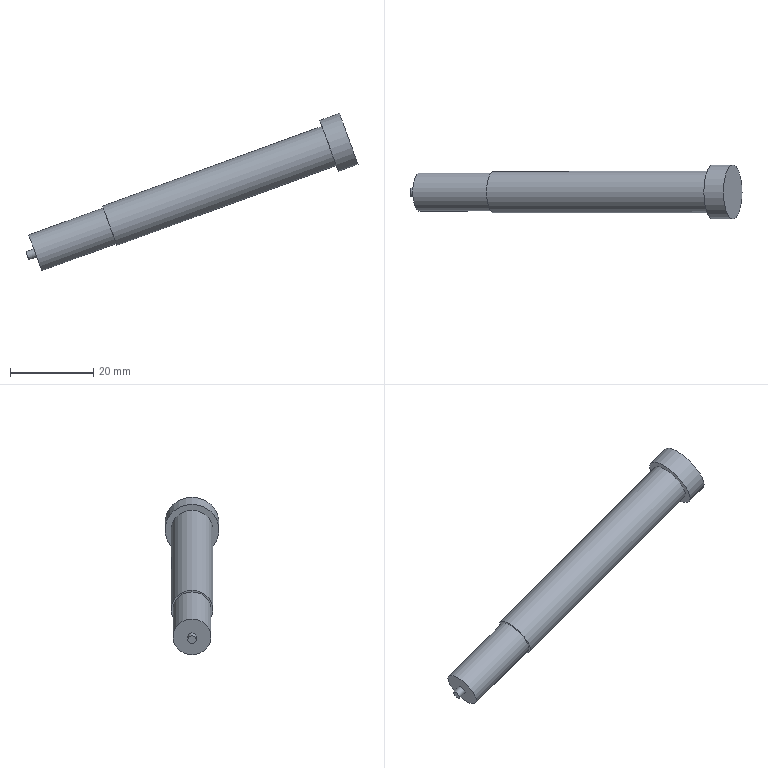Part | NX | features solid 2 | 1 solid | 9 faces | box 79.62 x 13 x 37.745 mm | volume 6304 mm3 | plane 5 | cylinder 4 | commonest cylinder face diameters 2 x1 9.1 x1 10 x1 13 x1
STEP:
#1=CARTESIAN_POINT('',(678.985,-306.988,36.091));
#2=VERTEX_POINT('',#1);
#3=CARTESIAN_POINT('',(680.695,-306.988,31.393));
#4=DIRECTION('',(-0.9397,0.000001517,-0.342));
#5=DIRECTION('',(-0.342,0.00000071,0.9397));
#6=AXIS2_PLACEMENT_3D('',#3,#4,#5);
#7=CIRCLE('',#6,5.);
#8=EDGE_CURVE('',#2,#2,#7,.T.);
#9=ORIENTED_EDGE('',*,*,#8,.F.);
#10=EDGE_LOOP('',(#9));
#11=FACE_BOUND('',#10,.T.);
#12=CARTESIAN_POINT('',(731.608,-306.989,55.244));
#13=VERTEX_POINT('',#12);
#14=CARTESIAN_POINT('',(733.318,-306.989,50.546));
#15=DIRECTION('',(-0.9397,0.000001517,-0.342));
#16=DIRECTION('',(-0.342,0.00000071,0.9397));
#17=AXIS2_PLACEMENT_3D('',#14,#15,#16);
#18=CIRCLE('',#17,5.);
#19=EDGE_CURVE('',#13,#13,#18,.T.);
#20=ORIENTED_EDGE('',*,*,#19,.T.);
#21=EDGE_LOOP('',(#20));
#22=FACE_BOUND('',#21,.T.);
#23=CARTESIAN_POINT('',(738.016,-306.989,52.256));
#24=DIRECTION('',(-0.9397,0.000001517,-0.342));
#25=DIRECTION('',(0.342,-0.00000071,-0.9397));
#26=AXIS2_PLACEMENT_3D('',#23,#24,#25);
#27=CYLINDRICAL_SURFACE('',#26,5.);
#28=ADVANCED_FACE('',(#11,#22),#27,.T.);
#29=CARTESIAN_POINT('',(679.139,-306.988,35.668));
#30=VERTEX_POINT('',#29);
#31=CARTESIAN_POINT('',(680.695,-306.988,31.393));
#32=DIRECTION('',(-0.9397,0.000001517,-0.342));
#33=DIRECTION('',(-0.342,0.00000071,0.9397));
#34=AXIS2_PLACEMENT_3D('',#31,#32,#33);
#35=CIRCLE('',#34,4.55);
#36=EDGE_CURVE('',#30,#30,#35,.T.);
#37=ORIENTED_EDGE('',*,*,#36,.F.);
#38=EDGE_LOOP('',(#37));
#39=FACE_BOUND('',#38,.T.);
#40=ORIENTED_EDGE('',*,*,#8,.T.);
#41=EDGE_LOOP('',(#40));
#42=FACE_BOUND('',#41,.T.);
#43=CARTESIAN_POINT('',(680.695,-306.988,31.393));
#44=DIRECTION('',(0.9397,-0.000001517,0.342));
#45=DIRECTION('',(-0.342,0.00000071,0.9397));
#46=AXIS2_PLACEMENT_3D('',#43,#44,#45);
#47=PLANE('',#46);
#48=ADVANCED_FACE('',(#39,#42),#47,.F.);
#49=CARTESIAN_POINT('',(731.095,-306.989,56.654));
#50=VERTEX_POINT('',#49);
#51=CARTESIAN_POINT('',(733.318,-306.989,50.546));
#52=DIRECTION('',(-0.9397,0.000001517,-0.342));
#53=DIRECTION('',(-0.342,0.00000071,0.9397));
#54=AXIS2_PLACEMENT_3D('',#51,#52,#53);
#55=CIRCLE('',#54,6.5);
#56=EDGE_CURVE('',#50,#50,#55,.T.);
#57=ORIENTED_EDGE('',*,*,#56,.T.);
#58=EDGE_LOOP('',(#57));
#59=FACE_BOUND('',#58,.T.);
#60=ORIENTED_EDGE('',*,*,#19,.F.);
#61=EDGE_LOOP('',(#60));
#62=FACE_BOUND('',#61,.T.);
#63=CARTESIAN_POINT('',(733.318,-306.989,50.546));
#64=DIRECTION('',(0.9397,-0.000001517,0.342));
#65=DIRECTION('',(-0.342,0.00000071,0.9397));
#66=AXIS2_PLACEMENT_3D('',#63,#64,#65);
#67=PLANE('',#66);
#68=ADVANCED_FACE('',(#59,#62),#67,.F.);
#69=ORIENTED_EDGE('',*,*,#56,.F.);
#70=EDGE_LOOP('',(#69));
#71=FACE_BOUND('',#70,.T.);
#72=CARTESIAN_POINT('',(735.793,-306.989,58.364));
#73=VERTEX_POINT('',#72);
#74=CARTESIAN_POINT('',(738.016,-306.989,52.256));
#75=DIRECTION('',(-0.9397,0.000001517,-0.342));
#76=DIRECTION('',(-0.342,0.00000071,0.9397));
#77=AXIS2_PLACEMENT_3D('',#74,#75,#76);
#78=CIRCLE('',#77,6.5);
#79=EDGE_CURVE('',#73,#73,#78,.T.);
#80=ORIENTED_EDGE('',*,*,#79,.T.);
#81=EDGE_LOOP('',(#80));
#82=FACE_BOUND('',#81,.T.);
#83=CARTESIAN_POINT('',(733.318,-306.989,50.546));
#84=DIRECTION('',(0.9397,-0.000001517,0.342));
#85=DIRECTION('',(-0.342,0.00000071,0.9397));
#86=AXIS2_PLACEMENT_3D('',#83,#84,#85);
#87=CYLINDRICAL_SURFACE('',#86,6.5);
#88=ADVANCED_FACE('',(#71,#82),#87,.T.);
#89=ORIENTED_EDGE('',*,*,#79,.F.);
#90=EDGE_LOOP('',(#89));
#91=FACE_BOUND('',#90,.T.);
#92=CARTESIAN_POINT('',(738.016,-306.989,52.256));
#93=DIRECTION('',(0.9397,-0.000001517,0.342));
#94=DIRECTION('',(-0.342,0.00000071,0.9397));
#95=AXIS2_PLACEMENT_3D('',#92,#93,#94);
#96=PLANE('',#95);
#97=ADVANCED_FACE('',(#91),#96,.T.);
#98=CARTESIAN_POINT('',(661.285,-306.988,29.17));
#99=VERTEX_POINT('',#98);
#100=CARTESIAN_POINT('',(662.841,-306.988,24.894));
#101=DIRECTION('',(-0.9397,0.000001517,-0.342));
#102=DIRECTION('',(-0.342,0.00000071,0.9397));
#103=AXIS2_PLACEMENT_3D('',#100,#101,#102);
#104=CIRCLE('',#103,4.55);
#105=EDGE_CURVE('',#99,#99,#104,.T.);
#106=ORIENTED_EDGE('',*,*,#105,.F.);
#107=EDGE_LOOP('',(#106));
#108=FACE_BOUND('',#107,.T.);
#109=ORIENTED_EDGE('',*,*,#36,.T.);
#110=EDGE_LOOP('',(#109));
#111=FACE_BOUND('',#110,.T.);
#112=CARTESIAN_POINT('',(662.841,-306.988,24.894));
#113=DIRECTION('',(0.9397,-0.000001517,0.342));
#114=DIRECTION('',(-0.342,0.00000071,0.9397));
#115=AXIS2_PLACEMENT_3D('',#112,#113,#114);
#116=CYLINDRICAL_SURFACE('',#115,4.55);
#117=ADVANCED_FACE('',(#108,#111),#116,.T.);
#118=CARTESIAN_POINT('',(662.499,-306.988,25.834));
#119=VERTEX_POINT('',#118);
#120=CARTESIAN_POINT('',(662.841,-306.988,24.894));
#121=DIRECTION('',(-0.9397,0.000001517,-0.342));
#122=DIRECTION('',(-0.342,0.00000071,0.9397));
#123=AXIS2_PLACEMENT_3D('',#120,#121,#122);
#124=CIRCLE('',#123,1.);
#125=EDGE_CURVE('',#119,#119,#124,.T.);
#126=ORIENTED_EDGE('',*,*,#125,.F.);
#127=EDGE_LOOP('',(#126));
#128=FACE_BOUND('',#127,.T.);
#129=ORIENTED_EDGE('',*,*,#105,.T.);
#130=EDGE_LOOP('',(#129));
#131=FACE_BOUND('',#130,.T.);
#132=CARTESIAN_POINT('',(662.841,-306.988,24.894));
#133=DIRECTION('',(0.9397,-0.000001517,0.342));
#134=DIRECTION('',(-0.342,0.00000071,0.9397));
#135=AXIS2_PLACEMENT_3D('',#132,#133,#134);
#136=PLANE('',#135);
#137=ADVANCED_FACE('',(#128,#131),#136,.F.);
#138=CARTESIAN_POINT('',(660.619,-306.988,25.15));
#139=VERTEX_POINT('',#138);
#140=CARTESIAN_POINT('',(660.961,-306.988,24.21));
#141=DIRECTION('',(-0.9397,0.000001517,-0.342));
#142=DIRECTION('',(-0.342,0.00000071,0.9397));
#143=AXIS2_PLACEMENT_3D('',#140,#141,#142);
#144=CIRCLE('',#143,1.);
#145=EDGE_CURVE('',#139,#139,#144,.T.);
#146=ORIENTED_EDGE('',*,*,#145,.F.);
#147=EDGE_LOOP('',(#146));
#148=FACE_BOUND('',#147,.T.);
#149=ORIENTED_EDGE('',*,*,#125,.T.);
#150=EDGE_LOOP('',(#149));
#151=FACE_BOUND('',#150,.T.);
#152=CARTESIAN_POINT('',(660.961,-306.988,24.21));
#153=DIRECTION('',(0.9397,-0.000001517,0.342));
#154=DIRECTION('',(-0.342,0.00000071,0.9397));
#155=AXIS2_PLACEMENT_3D('',#152,#153,#154);
#156=CYLINDRICAL_SURFACE('',#155,1.);
#157=ADVANCED_FACE('',(#148,#151),#156,.T.);
#158=ORIENTED_EDGE('',*,*,#145,.T.);
#159=EDGE_LOOP('',(#158));
#160=FACE_BOUND('',#159,.T.);
#161=CARTESIAN_POINT('',(660.961,-306.988,24.21));
#162=DIRECTION('',(0.9397,-0.000001517,0.342));
#163=DIRECTION('',(-0.342,0.00000071,0.9397));
#164=AXIS2_PLACEMENT_3D('',#161,#162,#163);
#165=PLANE('',#164);
#166=ADVANCED_FACE('',(#160),#165,.F.);
#167=CLOSED_SHELL('',(#28,#48,#68,#88,#97,#117,#137,#157,#166));
#168=MANIFOLD_SOLID_BREP('',#167);
#169=(LENGTH_UNIT()NAMED_UNIT(*)SI_UNIT(.MILLI.,.METRE.));
#170=UNCERTAINTY_MEASURE_WITH_UNIT(LENGTH_MEASURE(0.00001),#169,'','');
#171=(NAMED_UNIT(*)PLANE_ANGLE_UNIT()SI_UNIT($,.RADIAN.));
#172=(NAMED_UNIT(*)SI_UNIT($,.STERADIAN.)SOLID_ANGLE_UNIT());
#173=(GEOMETRIC_REPRESENTATION_CONTEXT(3)GLOBAL_UNCERTAINTY_ASSIGNED_CONTEXT((#170))GLOBAL_UNIT_ASSIGNED_CONTEXT((#169,#171,#172))REPRESENTATION_CONTEXT('',''));
#174=ADVANCED_BREP_SHAPE_REPRESENTATION('',(#168),#173);